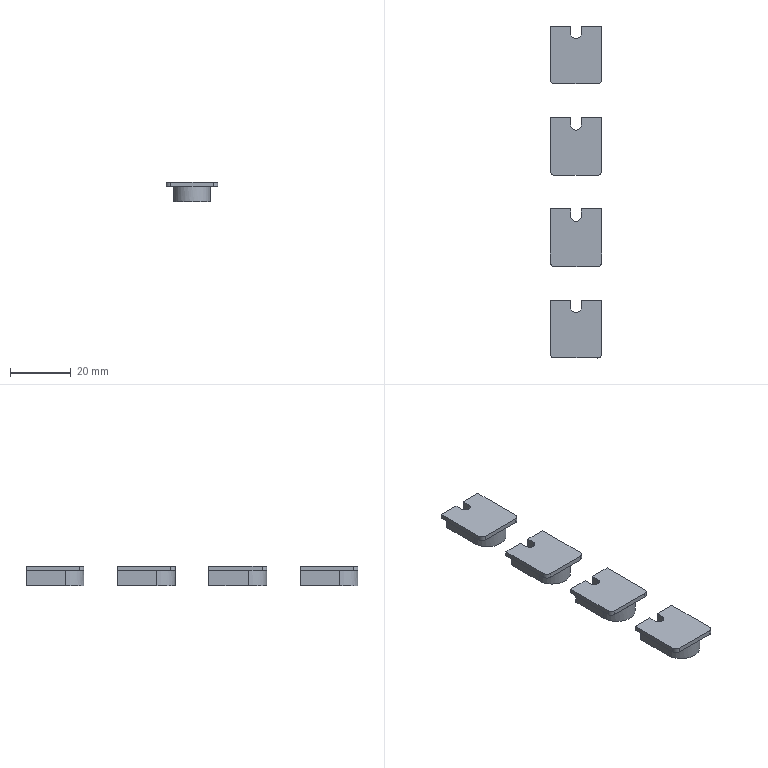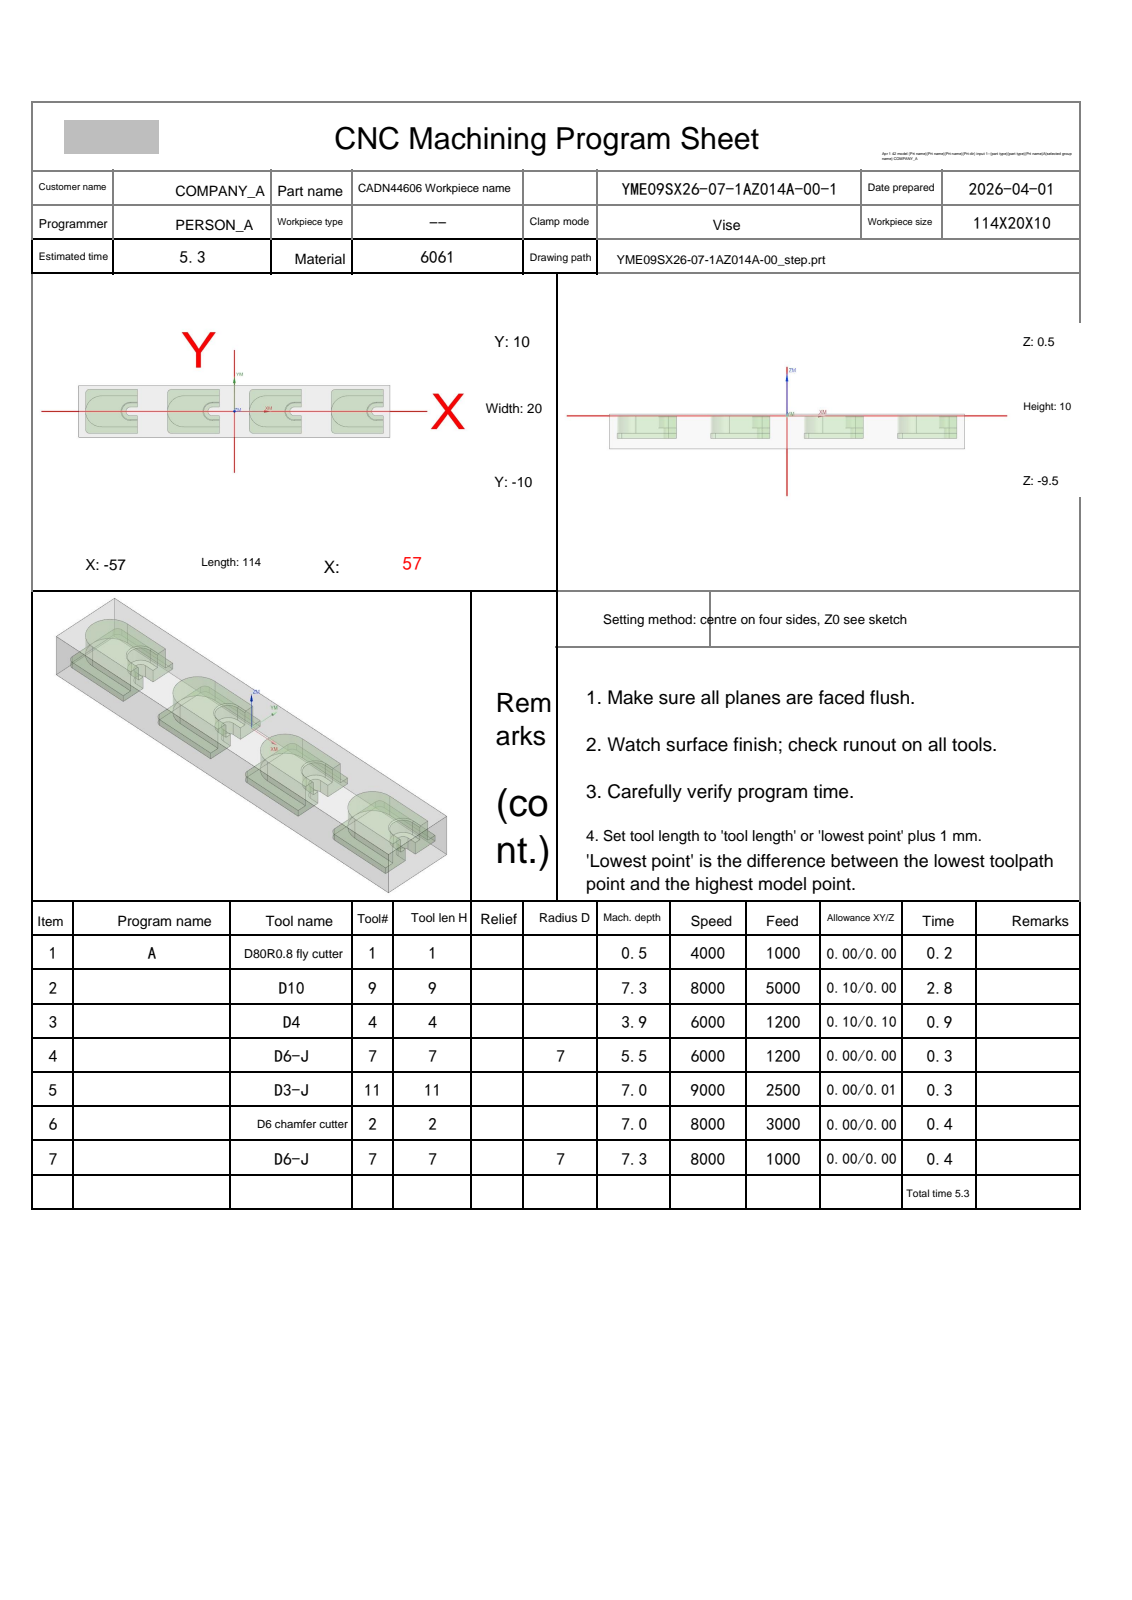NC program | NX | posted by the shop | part box 17.001 x 109 x 6.504 mm
Lines 1 to 2416 of 4321, first 1830 of 2414 lines:
%
O0001
(Machine time: 6.61 MIN)
(===Total Tool:6===)
(T1=D80R0.8 fly cutter D=80.  R=0.8  D-  H01 Z=-0.   )
(T9=D10     D=10.  R=0.   D-  H09 Z=-6.8  )
(T4=D4      D=4.   R=0.   D-  H04 Z=-3.4  )
(T7=D6-J    D=6.   R=0.   D7  H07 Z=-6.8  )
(T11=D3-J   D=3.   R=0.   D-  H11 Z=-6.45 )
(T2=D6 chamfer cutter   D=6.   R=0.   D-  H02 Z=-6.5  )
G80 G90 G17 G49 G40
G91 G28 Z0
M01
N1 T01 M06
(D80R0.8 fly cutter D=80. R=0.8 H=01 ce=0.00 di=0.00)
G00 G90 G54 X-99.5 Y.005 M03 S4000
G43 H01 Z20.
M08
Z2.
G01 Z0.0 F1000.
X-94.5
X94.5
X99.5
Z2.
G00 Z20.
G91 G28 Z0.0
M05
M09
G91 G28 Z0.0
M01
N2 T09 M06
(D10  D=10. R=0. H=09 ce=0.10 di=0.00)
G00 G90 G54 X15.75 Y13.6 M03 S8000
G43 H09 Z20.
M08
Z.5
G01 X24.5 Z.438 F5000.
G02 X29.6 Y8.5 Z.381 I0.0 J-5.1
G01 Y1.7 Z.333
G02 X29.308 Y0.0 Z.32 I-5.1 J0.0
X29.6 Y-1.7 Z.308 I-4.808 J-1.7
G01 Y-8.5 Z.26
G02 X24.5 Y-13.6 Z.203 I-5.1 J0.0
G01 X7. Z.079
G02 X.4 Y-7. Z.005 I0.0 J6.6
G01 Y7. Z-.094
G02 X7. Y13.6 Z-.168 I6.6 J0.0
G01 X24.5 Z-.292
G02 X29.6 Y8.5 Z-.349 I0.0 J-5.1
G01 Y1.7 Z-.397
G02 X29.308 Y0.0 Z-.41 I-5.1 J0.0
X29.6 Y-1.7 Z-.422 I-4.808 J-1.7
G01 Y-8.5 Z-.47
G02 X24.5 Y-13.6 Z-.527 I-5.1 J0.0
G01 X7. Z-.651
G02 X.4 Y-7. Z-.725 I0.0 J6.6
G01 Y7. Z-.824
G02 X7. Y13.6 Z-.898 I6.6 J0.0
G01 X24.5 Z-1.022
G02 X29.6 Y8.5 Z-1.079 I0.0 J-5.1
G01 Y1.7 Z-1.127
G02 X29.308 Y0.0 Z-1.14 I-5.1 J0.0
X29.6 Y-1.7 Z-1.152 I-4.808 J-1.7
G01 Y-8.5 Z-1.2
G02 X24.5 Y-13.6 Z-1.257 I-5.1 J0.0
G01 X7. Z-1.381
G02 X.4 Y-7. Z-1.455 I0.0 J6.6
G01 Y7. Z-1.554
G02 X7. Y13.6 Z-1.628 I6.6 J0.0
G01 X24.5 Z-1.752
G02 X29.6 Y8.5 Z-1.809 I0.0 J-5.1
G01 Y1.7 Z-1.857
G02 X29.308 Y0.0 Z-1.87 I-5.1 J0.0
X29.6 Y-1.7 Z-1.882 I-4.808 J-1.7
G01 Y-8.5 Z-1.93
G02 X24.5 Y-13.6 Z-1.987 I-5.1 J0.0
G01 X7. Z-2.111
G02 X.4 Y-7. Z-2.185 I0.0 J6.6
G01 Y7. Z-2.284
G02 X7. Y13.6 Z-2.358 I6.6 J0.0
G01 X24.5 Z-2.482
G02 X29.6 Y8.5 Z-2.539 I0.0 J-5.1
G01 Y1.7 Z-2.587
G02 X29.308 Y0.0 Z-2.6 I-5.1 J0.0
X29.6 Y-1.7 Z-2.612 I-4.808 J-1.7
G01 Y-8.5 Z-2.66
G02 X24.5 Y-13.6 Z-2.717 I-5.1 J0.0
G01 X7. Z-2.841
G02 X.4 Y-7. Z-2.915 I0.0 J6.6
G01 Y7. Z-3.014
G02 X7. Y13.6 Z-3.088 I6.6 J0.0
G01 X24.5 Z-3.212
G02 X29.6 Y8.5 Z-3.269 I0.0 J-5.1
G01 Y1.7 Z-3.317
G02 X29.308 Y0.0 Z-3.33 I-5.1 J0.0
X29.6 Y-1.7 Z-3.342 I-4.808 J-1.7
G01 Y-8.5 Z-3.39
G02 X24.5 Y-13.6 Z-3.447 I-5.1 J0.0
G01 X7. Z-3.571
G02 X.4 Y-7. Z-3.645 I0.0 J6.6
G01 Y7. Z-3.744
G02 X7. Y13.6 Z-3.818 I6.6 J0.0
G01 X24.5 Z-3.942
G02 X29.6 Y8.5 Z-3.999 I0.0 J-5.1
G01 Y1.7 Z-4.047
G02 X29.308 Y0.0 Z-4.06 I-5.1 J0.0
X29.6 Y-1.7 Z-4.072 I-4.808 J-1.7
G01 Y-8.5 Z-4.12
G02 X24.5 Y-13.6 Z-4.177 I-5.1 J0.0
G01 X7. Z-4.301
G02 X.4 Y-7. Z-4.375 I0.0 J6.6
G01 Y7. Z-4.474
G02 X7. Y13.6 Z-4.548 I6.6 J0.0
G01 X24.5 Z-4.672
G02 X29.6 Y8.5 Z-4.729 I0.0 J-5.1
G01 Y1.7 Z-4.777
G02 X29.308 Y0.0 Z-4.79 I-5.1 J0.0
X29.6 Y-1.7 Z-4.802 I-4.808 J-1.7
G01 Y-8.5 Z-4.85
G02 X24.5 Y-13.6 Z-4.907 I-5.1 J0.0
G01 X7. Z-5.031
G02 X.4 Y-7. Z-5.105 I0.0 J6.6
G01 Y7. Z-5.204
G02 X7. Y13.6 Z-5.278 I6.6 J0.0
G01 X24.5 Z-5.402
G02 X29.6 Y8.5 Z-5.459 I0.0 J-5.1
G01 Y1.7 Z-5.507
G02 X29.308 Y0.0 Z-5.52 I-5.1 J0.0
X29.6 Y-1.7 Z-5.532 I-4.808 J-1.7
G01 Y-8.5 Z-5.58
G02 X24.5 Y-13.6 Z-5.637 I-5.1 J0.0
G01 X7. Z-5.761
G02 X.4 Y-7. Z-5.835 I0.0 J6.6
G01 Y7. Z-5.934
G02 X7. Y13.6 Z-6.008 I6.6 J0.0
G01 X24.5 Z-6.132
G02 X29.6 Y8.5 Z-6.189 I0.0 J-5.1
G01 Y1.7 Z-6.237
G02 X29.308 Y0.0 Z-6.25 I-5.1 J0.0
X29.6 Y-1.7 Z-6.262 I-4.808 J-1.7
G01 Y-8.5 Z-6.31
G02 X24.5 Y-13.6 Z-6.367 I-5.1 J0.0
G01 X7. Z-6.491
G02 X.4 Y-7. Z-6.565 I0.0 J6.6
G01 Y7. Z-6.664
G02 X7. Y13.6 Z-6.738 I6.6 J0.0
G01 X15.75 Z-6.8
X24.5
G02 X29.6 Y8.5 I0.0 J-5.1
G01 Y1.7
G02 X29.308 Y0.0 I-5.1 J0.0
X29.6 Y-1.7 I-4.808 J-1.7
G01 Y-8.5
G02 X24.5 Y-13.6 I-5.1 J0.0
G01 X7.
G02 X.4 Y-7. I0.0 J6.6
G01 Y7.
G02 X7. Y13.6 I6.6 J0.0
G01 X15.75
X16.25
Z-5.8
G00 Z20.
X-14.25
Z.5
G01 X-5.5 Z.438
G02 X-.4 Y8.5 Z.381 I0.0 J-5.1
G01 Y1.7 Z.333
G02 X-.692 Y0.0 Z.32 I-5.1 J0.0
X-.4 Y-1.7 Z.308 I-4.808 J-1.7
G01 Y-8.5 Z.26
G02 X-5.5 Y-13.6 Z.203 I-5.1 J0.0
G01 X-23. Z.079
G02 X-29.6 Y-7. Z.005 I0.0 J6.6
G01 Y7. Z-.094
G02 X-23. Y13.6 Z-.168 I6.6 J0.0
G01 X-5.5 Z-.292
G02 X-.4 Y8.5 Z-.349 I0.0 J-5.1
G01 Y1.7 Z-.397
G02 X-.692 Y0.0 Z-.41 I-5.1 J0.0
X-.4 Y-1.7 Z-.422 I-4.808 J-1.7
G01 Y-8.5 Z-.47
G02 X-5.5 Y-13.6 Z-.527 I-5.1 J0.0
G01 X-23. Z-.651
G02 X-29.6 Y-7. Z-.725 I0.0 J6.6
G01 Y7. Z-.824
G02 X-23. Y13.6 Z-.898 I6.6 J0.0
G01 X-5.5 Z-1.022
G02 X-.4 Y8.5 Z-1.079 I0.0 J-5.1
G01 Y1.7 Z-1.127
G02 X-.692 Y0.0 Z-1.14 I-5.1 J0.0
X-.4 Y-1.7 Z-1.152 I-4.808 J-1.7
G01 Y-8.5 Z-1.2
G02 X-5.5 Y-13.6 Z-1.257 I-5.1 J0.0
G01 X-23. Z-1.381
G02 X-29.6 Y-7. Z-1.455 I0.0 J6.6
G01 Y7. Z-1.554
G02 X-23. Y13.6 Z-1.628 I6.6 J0.0
G01 X-5.5 Z-1.752
G02 X-.4 Y8.5 Z-1.809 I0.0 J-5.1
G01 Y1.7 Z-1.857
G02 X-.692 Y0.0 Z-1.87 I-5.1 J0.0
X-.4 Y-1.7 Z-1.882 I-4.808 J-1.7
G01 Y-8.5 Z-1.93
G02 X-5.5 Y-13.6 Z-1.987 I-5.1 J0.0
G01 X-23. Z-2.111
G02 X-29.6 Y-7. Z-2.185 I0.0 J6.6
G01 Y7. Z-2.284
G02 X-23. Y13.6 Z-2.358 I6.6 J0.0
G01 X-5.5 Z-2.482
G02 X-.4 Y8.5 Z-2.539 I0.0 J-5.1
G01 Y1.7 Z-2.587
G02 X-.692 Y0.0 Z-2.6 I-5.1 J0.0
X-.4 Y-1.7 Z-2.612 I-4.808 J-1.7
G01 Y-8.5 Z-2.66
G02 X-5.5 Y-13.6 Z-2.717 I-5.1 J0.0
G01 X-23. Z-2.841
G02 X-29.6 Y-7. Z-2.915 I0.0 J6.6
G01 Y7. Z-3.014
G02 X-23. Y13.6 Z-3.088 I6.6 J0.0
G01 X-5.5 Z-3.212
G02 X-.4 Y8.5 Z-3.269 I0.0 J-5.1
G01 Y1.7 Z-3.317
G02 X-.692 Y0.0 Z-3.33 I-5.1 J0.0
X-.4 Y-1.7 Z-3.342 I-4.808 J-1.7
G01 Y-8.5 Z-3.39
G02 X-5.5 Y-13.6 Z-3.447 I-5.1 J0.0
G01 X-23. Z-3.571
G02 X-29.6 Y-7. Z-3.645 I0.0 J6.6
G01 Y7. Z-3.744
G02 X-23. Y13.6 Z-3.818 I6.6 J0.0
G01 X-5.5 Z-3.942
G02 X-.4 Y8.5 Z-3.999 I0.0 J-5.1
G01 Y1.7 Z-4.047
G02 X-.692 Y0.0 Z-4.06 I-5.1 J0.0
X-.4 Y-1.7 Z-4.072 I-4.808 J-1.7
G01 Y-8.5 Z-4.12
G02 X-5.5 Y-13.6 Z-4.177 I-5.1 J0.0
G01 X-23. Z-4.301
G02 X-29.6 Y-7. Z-4.375 I0.0 J6.6
G01 Y7. Z-4.474
G02 X-23. Y13.6 Z-4.548 I6.6 J0.0
G01 X-5.5 Z-4.672
G02 X-.4 Y8.5 Z-4.729 I0.0 J-5.1
G01 Y1.7 Z-4.777
G02 X-.692 Y0.0 Z-4.79 I-5.1 J0.0
X-.4 Y-1.7 Z-4.802 I-4.808 J-1.7
G01 Y-8.5 Z-4.85
G02 X-5.5 Y-13.6 Z-4.907 I-5.1 J0.0
G01 X-23. Z-5.031
G02 X-29.6 Y-7. Z-5.105 I0.0 J6.6
G01 Y7. Z-5.204
G02 X-23. Y13.6 Z-5.278 I6.6 J0.0
G01 X-5.5 Z-5.402
G02 X-.4 Y8.5 Z-5.459 I0.0 J-5.1
G01 Y1.7 Z-5.507
G02 X-.692 Y0.0 Z-5.52 I-5.1 J0.0
X-.4 Y-1.7 Z-5.532 I-4.808 J-1.7
G01 Y-8.5 Z-5.58
G02 X-5.5 Y-13.6 Z-5.637 I-5.1 J0.0
G01 X-23. Z-5.761
G02 X-29.6 Y-7. Z-5.835 I0.0 J6.6
G01 Y7. Z-5.934
G02 X-23. Y13.6 Z-6.008 I6.6 J0.0
G01 X-5.5 Z-6.132
G02 X-.4 Y8.5 Z-6.189 I0.0 J-5.1
G01 Y1.7 Z-6.237
G02 X-.692 Y0.0 Z-6.25 I-5.1 J0.0
X-.4 Y-1.7 Z-6.262 I-4.808 J-1.7
G01 Y-8.5 Z-6.31
G02 X-5.5 Y-13.6 Z-6.367 I-5.1 J0.0
G01 X-23. Z-6.491
G02 X-29.6 Y-7. Z-6.565 I0.0 J6.6
G01 Y7. Z-6.664
G02 X-23. Y13.6 Z-6.738 I6.6 J0.0
G01 X-14.25 Z-6.8
X-5.5
G02 X-.4 Y8.5 I0.0 J-5.1
G01 Y1.7
G02 X-.692 Y0.0 I-5.1 J0.0
X-.4 Y-1.7 I-4.808 J-1.7
G01 Y-8.5
G02 X-5.5 Y-13.6 I-5.1 J0.0
G01 X-23.
G02 X-29.6 Y-7. I0.0 J6.6
G01 Y7.
G02 X-23. Y13.6 I6.6 J0.0
G01 X-14.25
X-13.75
Z-5.8
G00 Z20.
X-44.25
Z.5
G01 X-35.5 Z.438
G02 X-30.4 Y8.5 Z.381 I0.0 J-5.1
G01 Y1.7 Z.333
G02 X-30.692 Y0.0 Z.32 I-5.1 J0.0
X-30.4 Y-1.7 Z.308 I-4.808 J-1.7
G01 Y-8.5 Z.26
G02 X-35.5 Y-13.6 Z.203 I-5.1 J0.0
G01 X-53. Z.079
G02 X-59.6 Y-7. Z.005 I0.0 J6.6
G01 Y7. Z-.094
G02 X-53. Y13.6 Z-.168 I6.6 J0.0
G01 X-35.5 Z-.292
G02 X-30.4 Y8.5 Z-.349 I0.0 J-5.1
G01 Y1.7 Z-.397
G02 X-30.692 Y0.0 Z-.41 I-5.1 J0.0
X-30.4 Y-1.7 Z-.422 I-4.808 J-1.7
G01 Y-8.5 Z-.47
G02 X-35.5 Y-13.6 Z-.527 I-5.1 J0.0
G01 X-53. Z-.651
G02 X-59.6 Y-7. Z-.725 I0.0 J6.6
G01 Y7. Z-.824
G02 X-53. Y13.6 Z-.898 I6.6 J0.0
G01 X-35.5 Z-1.022
G02 X-30.4 Y8.5 Z-1.079 I0.0 J-5.1
G01 Y1.7 Z-1.127
G02 X-30.692 Y0.0 Z-1.14 I-5.1 J0.0
X-30.4 Y-1.7 Z-1.152 I-4.808 J-1.7
G01 Y-8.5 Z-1.2
G02 X-35.5 Y-13.6 Z-1.257 I-5.1 J0.0
G01 X-53. Z-1.381
G02 X-59.6 Y-7. Z-1.455 I0.0 J6.6
G01 Y7. Z-1.554
G02 X-53. Y13.6 Z-1.628 I6.6 J0.0
G01 X-35.5 Z-1.752
G02 X-30.4 Y8.5 Z-1.809 I0.0 J-5.1
G01 Y1.7 Z-1.857
G02 X-30.692 Y0.0 Z-1.87 I-5.1 J0.0
X-30.4 Y-1.7 Z-1.882 I-4.808 J-1.7
G01 Y-8.5 Z-1.93
G02 X-35.5 Y-13.6 Z-1.987 I-5.1 J0.0
G01 X-53. Z-2.111
G02 X-59.6 Y-7. Z-2.185 I0.0 J6.6
G01 Y7. Z-2.284
G02 X-53. Y13.6 Z-2.358 I6.6 J0.0
G01 X-35.5 Z-2.482
G02 X-30.4 Y8.5 Z-2.539 I0.0 J-5.1
G01 Y1.7 Z-2.587
G02 X-30.692 Y0.0 Z-2.6 I-5.1 J0.0
X-30.4 Y-1.7 Z-2.612 I-4.808 J-1.7
G01 Y-8.5 Z-2.66
G02 X-35.5 Y-13.6 Z-2.717 I-5.1 J0.0
G01 X-53. Z-2.841
G02 X-59.6 Y-7. Z-2.915 I0.0 J6.6
G01 Y7. Z-3.014
G02 X-53. Y13.6 Z-3.088 I6.6 J0.0
G01 X-35.5 Z-3.212
G02 X-30.4 Y8.5 Z-3.269 I0.0 J-5.1
G01 Y1.7 Z-3.317
G02 X-30.692 Y0.0 Z-3.33 I-5.1 J0.0
X-30.4 Y-1.7 Z-3.342 I-4.808 J-1.7
G01 Y-8.5 Z-3.39
G02 X-35.5 Y-13.6 Z-3.447 I-5.1 J0.0
G01 X-53. Z-3.571
G02 X-59.6 Y-7. Z-3.645 I0.0 J6.6
G01 Y7. Z-3.744
G02 X-53. Y13.6 Z-3.818 I6.6 J0.0
G01 X-35.5 Z-3.942
G02 X-30.4 Y8.5 Z-3.999 I0.0 J-5.1
G01 Y1.7 Z-4.047
G02 X-30.692 Y0.0 Z-4.06 I-5.1 J0.0
X-30.4 Y-1.7 Z-4.072 I-4.808 J-1.7
G01 Y-8.5 Z-4.12
G02 X-35.5 Y-13.6 Z-4.177 I-5.1 J0.0
G01 X-53. Z-4.301
G02 X-59.6 Y-7. Z-4.375 I0.0 J6.6
G01 Y7. Z-4.474
G02 X-53. Y13.6 Z-4.548 I6.6 J0.0
G01 X-35.5 Z-4.672
G02 X-30.4 Y8.5 Z-4.729 I0.0 J-5.1
G01 Y1.7 Z-4.777
G02 X-30.692 Y0.0 Z-4.79 I-5.1 J0.0
X-30.4 Y-1.7 Z-4.802 I-4.808 J-1.7
G01 Y-8.5 Z-4.85
G02 X-35.5 Y-13.6 Z-4.907 I-5.1 J0.0
G01 X-53. Z-5.031
G02 X-59.6 Y-7. Z-5.105 I0.0 J6.6
G01 Y7. Z-5.204
G02 X-53. Y13.6 Z-5.278 I6.6 J0.0
G01 X-35.5 Z-5.402
G02 X-30.4 Y8.5 Z-5.459 I0.0 J-5.1
G01 Y1.7 Z-5.507
G02 X-30.692 Y0.0 Z-5.52 I-5.1 J0.0
X-30.4 Y-1.7 Z-5.532 I-4.808 J-1.7
G01 Y-8.5 Z-5.58
G02 X-35.5 Y-13.6 Z-5.637 I-5.1 J0.0
G01 X-53. Z-5.761
G02 X-59.6 Y-7. Z-5.835 I0.0 J6.6
G01 Y7. Z-5.934
G02 X-53. Y13.6 Z-6.008 I6.6 J0.0
G01 X-35.5 Z-6.132
G02 X-30.4 Y8.5 Z-6.189 I0.0 J-5.1
G01 Y1.7 Z-6.237
G02 X-30.692 Y0.0 Z-6.25 I-5.1 J0.0
X-30.4 Y-1.7 Z-6.262 I-4.808 J-1.7
G01 Y-8.5 Z-6.31
G02 X-35.5 Y-13.6 Z-6.367 I-5.1 J0.0
G01 X-53. Z-6.491
G02 X-59.6 Y-7. Z-6.565 I0.0 J6.6
G01 Y7. Z-6.664
G02 X-53. Y13.6 Z-6.738 I6.6 J0.0
G01 X-44.25 Z-6.8
X-35.5
G02 X-30.4 Y8.5 I0.0 J-5.1
G01 Y1.7
G02 X-30.692 Y0.0 I-5.1 J0.0
X-30.4 Y-1.7 I-4.808 J-1.7
G01 Y-8.5
G02 X-35.5 Y-13.6 I-5.1 J0.0
G01 X-53.
G02 X-59.6 Y-7. I0.0 J6.6
G01 Y7.
G02 X-53. Y13.6 I6.6 J0.0
G01 X-44.25
X-43.75
Z-5.8
G00 Z20.
X45.75
Z.5
G01 X54.5 Z.438
G02 X59.6 Y8.5 Z.381 I0.0 J-5.1
G01 Y1.7 Z.333
G02 X59.308 Y0.0 Z.32 I-5.1 J0.0
X59.6 Y-1.7 Z.308 I-4.808 J-1.7
G01 Y-8.5 Z.26
G02 X54.5 Y-13.6 Z.203 I-5.1 J0.0
G01 X37. Z.079
G02 X30.4 Y-7. Z.005 I0.0 J6.6
G01 Y7. Z-.094
G02 X37. Y13.6 Z-.168 I6.6 J0.0
G01 X54.5 Z-.292
G02 X59.6 Y8.5 Z-.349 I0.0 J-5.1
G01 Y1.7 Z-.397
G02 X59.308 Y0.0 Z-.41 I-5.1 J0.0
X59.6 Y-1.7 Z-.422 I-4.808 J-1.7
G01 Y-8.5 Z-.47
G02 X54.5 Y-13.6 Z-.527 I-5.1 J0.0
G01 X37. Z-.651
G02 X30.4 Y-7. Z-.725 I0.0 J6.6
G01 Y7. Z-.824
G02 X37. Y13.6 Z-.898 I6.6 J0.0
G01 X54.5 Z-1.022
G02 X59.6 Y8.5 Z-1.079 I0.0 J-5.1
G01 Y1.7 Z-1.127
G02 X59.308 Y0.0 Z-1.14 I-5.1 J0.0
X59.6 Y-1.7 Z-1.152 I-4.808 J-1.7
G01 Y-8.5 Z-1.2
G02 X54.5 Y-13.6 Z-1.257 I-5.1 J0.0
G01 X37. Z-1.381
G02 X30.4 Y-7. Z-1.455 I0.0 J6.6
G01 Y7. Z-1.554
G02 X37. Y13.6 Z-1.628 I6.6 J0.0
G01 X54.5 Z-1.752
G02 X59.6 Y8.5 Z-1.809 I0.0 J-5.1
G01 Y1.7 Z-1.857
G02 X59.308 Y0.0 Z-1.87 I-5.1 J0.0
X59.6 Y-1.7 Z-1.882 I-4.808 J-1.7
G01 Y-8.5 Z-1.93
G02 X54.5 Y-13.6 Z-1.987 I-5.1 J0.0
G01 X37. Z-2.111
G02 X30.4 Y-7. Z-2.185 I0.0 J6.6
G01 Y7. Z-2.284
G02 X37. Y13.6 Z-2.358 I6.6 J0.0
G01 X54.5 Z-2.482
G02 X59.6 Y8.5 Z-2.539 I0.0 J-5.1
G01 Y1.7 Z-2.587
G02 X59.308 Y0.0 Z-2.6 I-5.1 J0.0
X59.6 Y-1.7 Z-2.612 I-4.808 J-1.7
G01 Y-8.5 Z-2.66
G02 X54.5 Y-13.6 Z-2.717 I-5.1 J0.0
G01 X37. Z-2.841
G02 X30.4 Y-7. Z-2.915 I0.0 J6.6
G01 Y7. Z-3.014
G02 X37. Y13.6 Z-3.088 I6.6 J0.0
G01 X54.5 Z-3.212
G02 X59.6 Y8.5 Z-3.269 I0.0 J-5.1
G01 Y1.7 Z-3.317
G02 X59.308 Y0.0 Z-3.33 I-5.1 J0.0
X59.6 Y-1.7 Z-3.342 I-4.808 J-1.7
G01 Y-8.5 Z-3.39
G02 X54.5 Y-13.6 Z-3.447 I-5.1 J0.0
G01 X37. Z-3.571
G02 X30.4 Y-7. Z-3.645 I0.0 J6.6
G01 Y7. Z-3.744
G02 X37. Y13.6 Z-3.818 I6.6 J0.0
G01 X54.5 Z-3.942
G02 X59.6 Y8.5 Z-3.999 I0.0 J-5.1
G01 Y1.7 Z-4.047
G02 X59.308 Y0.0 Z-4.06 I-5.1 J0.0
X59.6 Y-1.7 Z-4.072 I-4.808 J-1.7
G01 Y-8.5 Z-4.12
G02 X54.5 Y-13.6 Z-4.177 I-5.1 J0.0
G01 X37. Z-4.301
G02 X30.4 Y-7. Z-4.375 I0.0 J6.6
G01 Y7. Z-4.474
G02 X37. Y13.6 Z-4.548 I6.6 J0.0
G01 X54.5 Z-4.672
G02 X59.6 Y8.5 Z-4.729 I0.0 J-5.1
G01 Y1.7 Z-4.777
G02 X59.308 Y0.0 Z-4.79 I-5.1 J0.0
X59.6 Y-1.7 Z-4.802 I-4.808 J-1.7
G01 Y-8.5 Z-4.85
G02 X54.5 Y-13.6 Z-4.907 I-5.1 J0.0
G01 X37. Z-5.031
G02 X30.4 Y-7. Z-5.105 I0.0 J6.6
G01 Y7. Z-5.204
G02 X37. Y13.6 Z-5.278 I6.6 J0.0
G01 X54.5 Z-5.402
G02 X59.6 Y8.5 Z-5.459 I0.0 J-5.1
G01 Y1.7 Z-5.507
G02 X59.308 Y0.0 Z-5.52 I-5.1 J0.0
X59.6 Y-1.7 Z-5.532 I-4.808 J-1.7
G01 Y-8.5 Z-5.58
G02 X54.5 Y-13.6 Z-5.637 I-5.1 J0.0
G01 X37. Z-5.761
G02 X30.4 Y-7. Z-5.835 I0.0 J6.6
G01 Y7. Z-5.934
G02 X37. Y13.6 Z-6.008 I6.6 J0.0
G01 X54.5 Z-6.132
G02 X59.6 Y8.5 Z-6.189 I0.0 J-5.1
G01 Y1.7 Z-6.237
G02 X59.308 Y0.0 Z-6.25 I-5.1 J0.0
X59.6 Y-1.7 Z-6.262 I-4.808 J-1.7
G01 Y-8.5 Z-6.31
G02 X54.5 Y-13.6 Z-6.367 I-5.1 J0.0
G01 X37. Z-6.491
G02 X30.4 Y-7. Z-6.565 I0.0 J6.6
G01 Y7. Z-6.664
G02 X37. Y13.6 Z-6.738 I6.6 J0.0
G01 X45.75 Z-6.8
X54.5
G02 X59.6 Y8.5 I0.0 J-5.1
G01 Y1.7
G02 X59.308 Y0.0 I-5.1 J0.0
X59.6 Y-1.7 I-4.808 J-1.7
G01 Y-8.5
G02 X54.5 Y-13.6 I-5.1 J0.0
G01 X37.
G02 X30.4 Y-7. I0.0 J6.6
G01 Y7.
G02 X37. Y13.6 I6.6 J0.0
G01 X45.75
X46.25
Z-5.8
G00 Z20.
G00 G90 X-11.8 Y16.5 M03 S8000
Z10.5
Z.956
G01 Z-.544 F4000.
Y13.4
X-.6
Y13.291
X5.26 Y13.159
X5.275 Y13.163
G02 X7. Y13.4 I1.725 J-6.163
G01 X29.4
Y13.291
X35.26 Y13.159
X35.275 Y13.163
G02 X37. Y13.4 I1.725 J-6.163
G01 X59.4
Y11.1
X41.5
G03 X31.1 Y3.879 I0.0 J-11.1
G01 Y11.1
G03 X29.6 Y12.6 I-1.5 J0.0
G01 X11.5
G03 X1.1 Y7.113 I0.0 J-12.6
G01 Y11.1
G03 X-.4 Y12.6 I-1.5 J0.0
G01 X-18.5
G03 X-30.4 Y4.141 I0.0 J-12.6
G01 Y11.1
X-48.5
G03 X-59.4 Y2.098 I0.0 J-11.1
G01 Y4.899
Y7.
G02 X-53. Y13.4 I6.4 J0.0
G01 X-30.6
Y13.291
X-24.739 Y13.159
X-24.725 Y13.163
G02 X-23. Y13.4 I1.725 J-6.163
G01 X-11.8
X-11.3
Y16.5
Z.956
G00 Z10.5
X48.2 Y-16.5
Z.956
G01 Z-.544
Y-13.4
X37.
G02 X35.26 Y-13.159 I0.0 J6.4
G01 X29.4 Y-13.291
Y-13.4
X7.
G02 X5.26 Y-13.159 I0.0 J6.4
G01 X-.6 Y-13.291
Y-13.4
X-23.
G02 X-24.74 Y-13.159 I0.0 J6.4
G01 X-30.6 Y-13.291
Y-13.4
X-53.
G02 X-59.4 Y-7. I0.0 J6.4
G01 Y-4.903
Y-2.097
G03 X-48.5 Y-11.1 I10.9 J2.097
G01 X-30.4
Y-4.141
G03 X-18.5 Y-12.6 I11.9 J4.141
G01 X-.4
G03 X1.1 Y-11.1 I0.0 J1.5
G01 Y-7.641
G03 X.623 Y-6.887 I-.835 J0.0
G01 X.243 Y-6.707
X.05 Y-6.663
G03 X-.4 Y-7.113 I0.0 J-.45
G01 Y-11.1
X-18.5
G02 X-29.6 Y0.0 I0.0 J11.1
X-18.5 Y11.1 I11.1 J0.0
G01 X-.4
Y-7.113
G03 X.532 Y-8.045 I.932 J0.0
X.869 Y-7.982 I0.0 J.932
G02 X1.23 Y-7.915 I.361 J-.933
X1.984 Y-8.259 I0.0 J-1.
G03 X11.5 Y-12.6 I9.516 J8.259
G01 X29.6
G03 X31.1 Y-11.1 I0.0 J1.5
G01 Y-4.407
G03 X30.623 Y-3.653 I-.835 J0.0
G01 X30.243 Y-3.473
X30.05 Y-3.429
G03 X29.6 Y-3.879 I0.0 J-.45
G01 Y-11.1
X11.5
G02 X.4 Y0.0 I0.0 J11.1
X11.5 Y11.1 I11.1 J0.0
G01 X29.6
Y-3.879
G03 X29.774 Y-4.235 I.45 J0.0
X30.019 Y-4.319 I.245 J.316
X30.338 Y-4.161 I0.0 J.4
G01 X30.607 Y-3.807
G02 X30.833 Y-3.694 I.227 J-.172
X31.1 Y-3.879 I0.0 J-.285
G03 X41.5 Y-11.1 I10.4 J3.879
G01 X59.4
Y-13.4
X48.2
X47.7
Y-16.5
Z.956
G00 Z10.5
X-11.8 Y16.5
Z.411
G01 Z-1.089
Y13.4
X-.6
Y13.291
X5.26 Y13.159
X5.275 Y13.163
G02 X7. Y13.4 I1.725 J-6.163
G01 X29.4
Y13.291
X35.26 Y13.159
X35.275 Y13.163
G02 X37. Y13.4 I1.725 J-6.163
G01 X59.4
Y11.1
X41.5
G03 X31.1 Y3.879 I0.0 J-11.1
G01 Y11.1
G03 X29.6 Y12.6 I-1.5 J0.0
G01 X11.5
G03 X1.1 Y7.113 I0.0 J-12.6
G01 Y11.1
G03 X-.4 Y12.6 I-1.5 J0.0
G01 X-18.5
G03 X-30.4 Y4.141 I0.0 J-12.6
G01 Y11.1
X-48.5
G03 X-59.4 Y2.098 I0.0 J-11.1
G01 Y4.899
Y7.
G02 X-53. Y13.4 I6.4 J0.0
G01 X-30.6
Y13.291
X-24.739 Y13.159
X-24.725 Y13.163
G02 X-23. Y13.4 I1.725 J-6.163
G01 X-11.8
X-11.3
Y16.5
Z.411
G00 Z10.5
X48.2 Y-16.5
Z.411
G01 Z-1.089
Y-13.4
X37.
G02 X35.26 Y-13.159 I0.0 J6.4
G01 X29.4 Y-13.291
Y-13.4
X7.
G02 X5.26 Y-13.159 I0.0 J6.4
G01 X-.6 Y-13.291
Y-13.4
X-23.
G02 X-24.74 Y-13.159 I0.0 J6.4
G01 X-30.6 Y-13.291
Y-13.4
X-53.
G02 X-59.4 Y-7. I0.0 J6.4
G01 Y-4.903
Y-2.097
G03 X-48.5 Y-11.1 I10.9 J2.097
G01 X-30.4
Y-4.141
G03 X-18.5 Y-12.6 I11.9 J4.141
G01 X-.4
G03 X1.1 Y-11.1 I0.0 J1.5
G01 Y-7.641
G03 X.623 Y-6.887 I-.835 J0.0
G01 X.243 Y-6.707
X.05 Y-6.663
G03 X-.4 Y-7.113 I0.0 J-.45
G01 Y-11.1
X-18.5
G02 X-29.6 Y0.0 I0.0 J11.1
X-18.5 Y11.1 I11.1 J0.0
G01 X-.4
Y-7.113
G03 X.532 Y-8.045 I.932 J0.0
X.869 Y-7.982 I0.0 J.932
G02 X1.23 Y-7.915 I.361 J-.933
X1.984 Y-8.259 I0.0 J-1.
G03 X11.5 Y-12.6 I9.516 J8.259
G01 X29.6
G03 X31.1 Y-11.1 I0.0 J1.5
G01 Y-4.407
G03 X30.623 Y-3.653 I-.835 J0.0
G01 X30.243 Y-3.473
X30.05 Y-3.429
G03 X29.6 Y-3.879 I0.0 J-.45
G01 Y-11.1
X11.5
G02 X.4 Y0.0 I0.0 J11.1
X11.5 Y11.1 I11.1 J0.0
G01 X29.6
Y-3.879
G03 X29.774 Y-4.235 I.45 J0.0
X30.019 Y-4.319 I.245 J.316
X30.338 Y-4.161 I0.0 J.4
G01 X30.607 Y-3.807
G02 X30.833 Y-3.694 I.227 J-.172
X31.1 Y-3.879 I0.0 J-.285
G03 X41.5 Y-11.1 I10.4 J3.879
G01 X59.4
Y-13.4
X48.2
X47.7
Y-16.5
Z.411
G00 Z10.5
X-11.8 Y16.5
Z-.133
G01 Z-1.633
Y13.4
X-.6
Y13.291
X5.26 Y13.159
X5.275 Y13.163
G02 X7. Y13.4 I1.725 J-6.163
G01 X29.4
Y13.291
X35.26 Y13.159
X35.275 Y13.163
G02 X37. Y13.4 I1.725 J-6.163
G01 X59.4
Y11.1
X41.5
G03 X31.1 Y3.879 I0.0 J-11.1
G01 Y11.1
G03 X29.6 Y12.6 I-1.5 J0.0
G01 X11.5
G03 X1.1 Y7.113 I0.0 J-12.6
G01 Y11.1
G03 X-.4 Y12.6 I-1.5 J0.0
G01 X-18.5
G03 X-30.4 Y4.141 I0.0 J-12.6
G01 Y11.1
X-48.5
G03 X-59.4 Y2.098 I0.0 J-11.1
G01 Y4.899
Y7.
G02 X-53. Y13.4 I6.4 J0.0
G01 X-30.6
Y13.291
X-24.739 Y13.159
X-24.725 Y13.163
G02 X-23. Y13.4 I1.725 J-6.163
G01 X-11.8
X-11.3
Y16.5
Z-.133
G00 Z10.5
X48.2 Y-16.5
Z-.133
G01 Z-1.633
Y-13.4
X37.
G02 X35.26 Y-13.159 I0.0 J6.4
G01 X29.4 Y-13.291
Y-13.4
X7.
G02 X5.26 Y-13.159 I0.0 J6.4
G01 X-.6 Y-13.291
Y-13.4
X-23.
G02 X-24.74 Y-13.159 I0.0 J6.4
G01 X-30.6 Y-13.291
Y-13.4
X-53.
G02 X-59.4 Y-7. I0.0 J6.4
G01 Y-4.903
Y-2.097
G03 X-48.5 Y-11.1 I10.9 J2.097
G01 X-30.4
Y-4.141
G03 X-18.5 Y-12.6 I11.9 J4.141
G01 X-.4
G03 X1.1 Y-11.1 I0.0 J1.5
G01 Y-7.641
G03 X.623 Y-6.887 I-.835 J0.0
G01 X.243 Y-6.707
X.05 Y-6.663
G03 X-.4 Y-7.113 I0.0 J-.45
G01 Y-11.1
X-18.5
G02 X-29.6 Y0.0 I0.0 J11.1
X-18.5 Y11.1 I11.1 J0.0
G01 X-.4
Y-7.113
G03 X.532 Y-8.045 I.932 J0.0
X.869 Y-7.982 I0.0 J.932
G02 X1.23 Y-7.915 I.361 J-.933
X1.984 Y-8.259 I0.0 J-1.
G03 X11.5 Y-12.6 I9.516 J8.259
G01 X29.6
G03 X31.1 Y-11.1 I0.0 J1.5
G01 Y-4.407
G03 X30.623 Y-3.653 I-.835 J0.0
G01 X30.243 Y-3.473
X30.05 Y-3.429
G03 X29.6 Y-3.879 I0.0 J-.45
G01 Y-11.1
X11.5
G02 X.4 Y0.0 I0.0 J11.1
X11.5 Y11.1 I11.1 J0.0
G01 X29.6
Y-3.879
G03 X29.774 Y-4.235 I.45 J0.0
X30.019 Y-4.319 I.245 J.316
X30.338 Y-4.161 I0.0 J.4
G01 X30.607 Y-3.807
G02 X30.833 Y-3.694 I.227 J-.172
X31.1 Y-3.879 I0.0 J-.285
G03 X41.5 Y-11.1 I10.4 J3.879
G01 X59.4
Y-13.4
X48.2
X47.7
Y-16.5
Z-.133
G00 Z10.5
X-11.8 Y16.5
Z-.678
G01 Z-2.178
Y13.4
X-.6
Y13.291
X5.26 Y13.159
X5.275 Y13.163
G02 X7. Y13.4 I1.725 J-6.163
G01 X29.4
Y13.291
X35.26 Y13.159
X35.275 Y13.163
G02 X37. Y13.4 I1.725 J-6.163
G01 X59.4
Y11.1
X41.5
G03 X31.1 Y3.879 I0.0 J-11.1
G01 Y11.1
G03 X29.6 Y12.6 I-1.5 J0.0
G01 X11.5
G03 X1.1 Y7.113 I0.0 J-12.6
G01 Y11.1
G03 X-.4 Y12.6 I-1.5 J0.0
G01 X-18.5
G03 X-30.4 Y4.141 I0.0 J-12.6
G01 Y11.1
X-48.5
G03 X-59.4 Y2.098 I0.0 J-11.1
G01 Y4.899
Y7.
G02 X-53. Y13.4 I6.4 J0.0
G01 X-30.6
Y13.291
X-24.739 Y13.159
X-24.725 Y13.163
G02 X-23. Y13.4 I1.725 J-6.163
G01 X-11.8
X-11.3
Y16.5
Z-.678
G00 Z10.5
X48.2 Y-16.5
Z-.678
G01 Z-2.178
Y-13.4
X37.
G02 X35.26 Y-13.159 I0.0 J6.4
G01 X29.4 Y-13.291
Y-13.4
X7.
G02 X5.26 Y-13.159 I0.0 J6.4
G01 X-.6 Y-13.291
Y-13.4
X-23.
G02 X-24.74 Y-13.159 I0.0 J6.4
G01 X-30.6 Y-13.291
Y-13.4
X-53.
G02 X-59.4 Y-7. I0.0 J6.4
G01 Y-4.903
Y-2.097
G03 X-48.5 Y-11.1 I10.9 J2.097
G01 X-30.4
Y-4.141
G03 X-18.5 Y-12.6 I11.9 J4.141
G01 X-.4
G03 X1.1 Y-11.1 I0.0 J1.5
G01 Y-7.641
G03 X.623 Y-6.887 I-.835 J0.0
G01 X.243 Y-6.707
X.05 Y-6.663
G03 X-.4 Y-7.113 I0.0 J-.45
G01 Y-11.1
X-18.5
G02 X-29.6 Y0.0 I0.0 J11.1
X-18.5 Y11.1 I11.1 J0.0
G01 X-.4
Y-7.113
G03 X.532 Y-8.045 I.932 J0.0
X.869 Y-7.982 I0.0 J.932
G02 X1.23 Y-7.915 I.361 J-.933
X1.984 Y-8.259 I0.0 J-1.
G03 X11.5 Y-12.6 I9.516 J8.259
G01 X29.6
G03 X31.1 Y-11.1 I0.0 J1.5
G01 Y-4.407
G03 X30.623 Y-3.653 I-.835 J0.0
G01 X30.243 Y-3.473
X30.05 Y-3.429
G03 X29.6 Y-3.879 I0.0 J-.45
G01 Y-11.1
X11.5
G02 X.4 Y0.0 I0.0 J11.1
X11.5 Y11.1 I11.1 J0.0
G01 X29.6
Y-3.879
G03 X29.774 Y-4.235 I.45 J0.0
X30.019 Y-4.319 I.245 J.316
X30.338 Y-4.161 I0.0 J.4
G01 X30.607 Y-3.807
G02 X30.833 Y-3.694 I.227 J-.172
X31.1 Y-3.879 I0.0 J-.285
G03 X41.5 Y-11.1 I10.4 J3.879
G01 X59.4
Y-13.4
X48.2
X47.7
Y-16.5
Z-.678
G00 Z10.5
X-11.8 Y16.5
Z-1.222
G01 Z-2.722
Y13.4
X-.6
Y13.291
X5.26 Y13.159
X5.275 Y13.163
G02 X7. Y13.4 I1.725 J-6.163
G01 X29.4
Y13.291
X35.26 Y13.159
X35.275 Y13.163
G02 X37. Y13.4 I1.725 J-6.163
G01 X59.4
Y11.1
X41.5
G03 X31.1 Y3.879 I0.0 J-11.1
G01 Y11.1
G03 X29.6 Y12.6 I-1.5 J0.0
G01 X11.5
G03 X1.1 Y7.113 I0.0 J-12.6
G01 Y11.1
G03 X-.4 Y12.6 I-1.5 J0.0
G01 X-18.5
G03 X-30.4 Y4.141 I0.0 J-12.6
G01 Y11.1
X-48.5
G03 X-59.4 Y2.098 I0.0 J-11.1
G01 Y4.899
Y7.
G02 X-53. Y13.4 I6.4 J0.0
G01 X-30.6
Y13.291
X-24.739 Y13.159
X-24.725 Y13.163
G02 X-23. Y13.4 I1.725 J-6.163
G01 X-11.8
X-11.3
Y16.5
Z-1.222
G00 Z10.5
X48.2 Y-16.5
Z-1.222
G01 Z-2.722
Y-13.4
X37.
G02 X35.26 Y-13.159 I0.0 J6.4
G01 X29.4 Y-13.291
Y-13.4
X7.
G02 X5.26 Y-13.159 I0.0 J6.4
G01 X-.6 Y-13.291
Y-13.4
X-23.
G02 X-24.74 Y-13.159 I0.0 J6.4
G01 X-30.6 Y-13.291
Y-13.4
X-53.
G02 X-59.4 Y-7. I0.0 J6.4
G01 Y-4.903
Y-2.097
G03 X-48.5 Y-11.1 I10.9 J2.097
G01 X-30.4
Y-4.141
G03 X-18.5 Y-12.6 I11.9 J4.141
G01 X-.4
G03 X1.1 Y-11.1 I0.0 J1.5
G01 Y-7.641
G03 X.623 Y-6.887 I-.835 J0.0
G01 X.243 Y-6.707
X.05 Y-6.663
G03 X-.4 Y-7.113 I0.0 J-.45
G01 Y-11.1
X-18.5
G02 X-29.6 Y0.0 I0.0 J11.1
X-18.5 Y11.1 I11.1 J0.0
G01 X-.4
Y-7.113
G03 X.532 Y-8.045 I.932 J0.0
X.869 Y-7.982 I0.0 J.932
G02 X1.23 Y-7.915 I.361 J-.933
X1.984 Y-8.259 I0.0 J-1.
G03 X11.5 Y-12.6 I9.516 J8.259
G01 X29.6
G03 X31.1 Y-11.1 I0.0 J1.5
G01 Y-4.407
G03 X30.623 Y-3.653 I-.835 J0.0
G01 X30.243 Y-3.473
X30.05 Y-3.429
G03 X29.6 Y-3.879 I0.0 J-.45
G01 Y-11.1
X11.5
G02 X.4 Y0.0 I0.0 J11.1
X11.5 Y11.1 I11.1 J0.0
G01 X29.6
Y-3.879
G03 X29.774 Y-4.235 I.45 J0.0
X30.019 Y-4.319 I.245 J.316
X30.338 Y-4.161 I0.0 J.4
G01 X30.607 Y-3.807
G02 X30.833 Y-3.694 I.227 J-.172
X31.1 Y-3.879 I0.0 J-.285
G03 X41.5 Y-11.1 I10.4 J3.879
G01 X59.4
Y-13.4
X48.2
X47.7
Y-16.5
Z-1.222
G00 Z10.5
X-11.8 Y16.5
Z-1.767
G01 Z-3.267
Y13.4
X-.6
Y13.291
X5.26 Y13.159
X5.275 Y13.163
G02 X7. Y13.4 I1.725 J-6.163
G01 X29.4
Y13.291
X35.26 Y13.159
X35.275 Y13.163
G02 X37. Y13.4 I1.725 J-6.163
G01 X59.4
Y11.1
X41.5
G03 X31.1 Y3.879 I0.0 J-11.1
G01 Y11.1
G03 X29.6 Y12.6 I-1.5 J0.0
G01 X11.5
G03 X1.1 Y7.113 I0.0 J-12.6
G01 Y11.1
G03 X-.4 Y12.6 I-1.5 J0.0
G01 X-18.5
G03 X-30.4 Y4.141 I0.0 J-12.6
G01 Y11.1
X-48.5
G03 X-59.4 Y2.098 I0.0 J-11.1
G01 Y4.899
Y7.
G02 X-53. Y13.4 I6.4 J0.0
G01 X-30.6
Y13.291
X-24.739 Y13.159
X-24.725 Y13.163
G02 X-23. Y13.4 I1.725 J-6.163
G01 X-11.8
X-11.3
Y16.5
Z-1.767
G00 Z10.5
X48.2 Y-16.5
Z-1.767
G01 Z-3.267
Y-13.4
X37.
G02 X35.26 Y-13.159 I0.0 J6.4
G01 X29.4 Y-13.291
Y-13.4
X7.
G02 X5.26 Y-13.159 I0.0 J6.4
G01 X-.6 Y-13.291
Y-13.4
X-23.
G02 X-24.74 Y-13.159 I0.0 J6.4
G01 X-30.6 Y-13.291
Y-13.4
X-53.
G02 X-59.4 Y-7. I0.0 J6.4
G01 Y-4.903
Y-2.097
G03 X-48.5 Y-11.1 I10.9 J2.097
G01 X-30.4
Y-4.141
G03 X-18.5 Y-12.6 I11.9 J4.141
G01 X-.4
G03 X1.1 Y-11.1 I0.0 J1.5
G01 Y-7.641
G03 X.623 Y-6.887 I-.835 J0.0
G01 X.243 Y-6.707
X.05 Y-6.663
G03 X-.4 Y-7.113 I0.0 J-.45
G01 Y-11.1
X-18.5
G02 X-29.6 Y0.0 I0.0 J11.1
X-18.5 Y11.1 I11.1 J0.0
G01 X-.4
Y-7.113
G03 X.532 Y-8.045 I.932 J0.0
X.869 Y-7.982 I0.0 J.932
G02 X1.23 Y-7.915 I.361 J-.933
X1.984 Y-8.259 I0.0 J-1.
G03 X11.5 Y-12.6 I9.516 J8.259
G01 X29.6
G03 X31.1 Y-11.1 I0.0 J1.5
G01 Y-4.407
G03 X30.623 Y-3.653 I-.835 J0.0
G01 X30.243 Y-3.473
X30.05 Y-3.429
G03 X29.6 Y-3.879 I0.0 J-.45
G01 Y-11.1
X11.5
G02 X.4 Y0.0 I0.0 J11.1
X11.5 Y11.1 I11.1 J0.0
G01 X29.6
Y-3.879
G03 X29.774 Y-4.235 I.45 J0.0
X30.019 Y-4.319 I.245 J.316
X30.338 Y-4.161 I0.0 J.4
G01 X30.607 Y-3.807
G02 X30.833 Y-3.694 I.227 J-.172
X31.1 Y-3.879 I0.0 J-.285
G03 X41.5 Y-11.1 I10.4 J3.879
G01 X59.4
Y-13.4
X48.2
X47.7
Y-16.5
Z-1.767
G00 Z10.5
X-11.8 Y16.5
Z-2.311
G01 Z-3.811
Y13.4
X-.6
Y13.291
X5.26 Y13.159
X5.275 Y13.163
G02 X7. Y13.4 I1.725 J-6.163
G01 X29.4
Y13.291
X35.26 Y13.159
X35.275 Y13.163
G02 X37. Y13.4 I1.725 J-6.163
G01 X59.4
Y11.1
X41.5
G03 X31.1 Y3.879 I0.0 J-11.1
G01 Y11.1
G03 X29.6 Y12.6 I-1.5 J0.0
G01 X11.5
G03 X1.1 Y7.113 I0.0 J-12.6
G01 Y11.1
G03 X-.4 Y12.6 I-1.5 J0.0
G01 X-18.5
G03 X-30.4 Y4.141 I0.0 J-12.6
G01 Y11.1
X-48.5
G03 X-59.4 Y2.098 I0.0 J-11.1
G01 Y4.899
Y7.
G02 X-53. Y13.4 I6.4 J0.0
G01 X-30.6
Y13.291
X-24.739 Y13.159
X-24.725 Y13.163
G02 X-23. Y13.4 I1.725 J-6.163
G01 X-11.8
X-11.3
Y16.5
Z-2.311
G00 Z10.5
X48.2 Y-16.5
Z-2.311
G01 Z-3.811
Y-13.4
X37.
G02 X35.26 Y-13.159 I0.0 J6.4
G01 X29.4 Y-13.291
Y-13.4
X7.
G02 X5.26 Y-13.159 I0.0 J6.4
G01 X-.6 Y-13.291
Y-13.4
X-23.
G02 X-24.74 Y-13.159 I0.0 J6.4
G01 X-30.6 Y-13.291
Y-13.4
X-53.
G02 X-59.4 Y-7. I0.0 J6.4
G01 Y-4.903
Y-2.097
G03 X-48.5 Y-11.1 I10.9 J2.097
G01 X-30.4
Y-4.141
G03 X-18.5 Y-12.6 I11.9 J4.141
G01 X-.4
G03 X1.1 Y-11.1 I0.0 J1.5
G01 Y-7.641
G03 X.623 Y-6.887 I-.835 J0.0
G01 X.243 Y-6.707
X.05 Y-6.663
G03 X-.4 Y-7.113 I0.0 J-.45
G01 Y-11.1
X-18.5
G02 X-29.6 Y0.0 I0.0 J11.1
X-18.5 Y11.1 I11.1 J0.0
G01 X-.4
Y-7.113
G03 X.532 Y-8.045 I.932 J0.0
X.869 Y-7.982 I0.0 J.932
G02 X1.23 Y-7.915 I.361 J-.933
X1.984 Y-8.259 I0.0 J-1.
G03 X11.5 Y-12.6 I9.516 J8.259
G01 X29.6
G03 X31.1 Y-11.1 I0.0 J1.5
G01 Y-4.407
G03 X30.623 Y-3.653 I-.835 J0.0
G01 X30.243 Y-3.473
X30.05 Y-3.429
G03 X29.6 Y-3.879 I0.0 J-.45
G01 Y-11.1
X11.5
G02 X.4 Y0.0 I0.0 J11.1
X11.5 Y11.1 I11.1 J0.0
G01 X29.6
Y-3.879
G03 X29.774 Y-4.235 I.45 J0.0
X30.019 Y-4.319 I.245 J.316
X30.338 Y-4.161 I0.0 J.4
G01 X30.607 Y-3.807
G02 X30.833 Y-3.694 I.227 J-.172
X31.1 Y-3.879 I0.0 J-.285
G03 X41.5 Y-11.1 I10.4 J3.879
G01 X59.4
Y-13.4
X48.2
X47.7
Y-16.5
Z-2.311
G00 Z10.5
X-11.8 Y16.5
Z-2.856
G01 Z-4.356
Y13.4
X-.6
Y13.291
X5.26 Y13.159
X5.275 Y13.163
G02 X7. Y13.4 I1.725 J-6.163
G01 X29.4
Y13.291
X35.26 Y13.159
X35.275 Y13.163
G02 X37. Y13.4 I1.725 J-6.163
G01 X59.4
Y11.1
X41.5
G03 X31.1 Y3.879 I0.0 J-11.1
G01 Y11.1
G03 X29.6 Y12.6 I-1.5 J0.0
G01 X11.5
G03 X1.1 Y7.113 I0.0 J-12.6
G01 Y11.1
G03 X-.4 Y12.6 I-1.5 J0.0
G01 X-18.5
G03 X-30.4 Y4.141 I0.0 J-12.6
G01 Y11.1
X-48.5
G03 X-59.4 Y2.098 I0.0 J-11.1
G01 Y4.899
Y7.
G02 X-53. Y13.4 I6.4 J0.0
G01 X-30.6
Y13.291
X-24.739 Y13.159
X-24.725 Y13.163
G02 X-23. Y13.4 I1.725 J-6.163
G01 X-11.8
X-11.3
Y16.5
Z-2.856
G00 Z10.5
X48.2 Y-16.5
Z-2.856
G01 Z-4.356
Y-13.4
X37.
G02 X35.26 Y-13.159 I0.0 J6.4
G01 X29.4 Y-13.291
Y-13.4
X7.
G02 X5.26 Y-13.159 I0.0 J6.4
G01 X-.6 Y-13.291
Y-13.4
X-23.
G02 X-24.74 Y-13.159 I0.0 J6.4
G01 X-30.6 Y-13.291
Y-13.4
X-53.
G02 X-59.4 Y-7. I0.0 J6.4
G01 Y-4.903
Y-2.097
G03 X-48.5 Y-11.1 I10.9 J2.097
G01 X-30.4
Y-4.141
G03 X-18.5 Y-12.6 I11.9 J4.141
G01 X-.4
G03 X1.1 Y-11.1 I0.0 J1.5
G01 Y-7.641
G03 X.623 Y-6.887 I-.835 J0.0
G01 X.243 Y-6.707
X.05 Y-6.663
G03 X-.4 Y-7.113 I0.0 J-.45
G01 Y-11.1
X-18.5
G02 X-29.6 Y0.0 I0.0 J11.1
X-18.5 Y11.1 I11.1 J0.0
G01 X-.4
Y-7.113
G03 X.532 Y-8.045 I.932 J0.0
X.869 Y-7.982 I0.0 J.932
G02 X1.23 Y-7.915 I.361 J-.933
X1.984 Y-8.259 I0.0 J-1.
G03 X11.5 Y-12.6 I9.516 J8.259
G01 X29.6
G03 X31.1 Y-11.1 I0.0 J1.5
G01 Y-4.407
G03 X30.623 Y-3.653 I-.835 J0.0
G01 X30.243 Y-3.473
X30.05 Y-3.429
G03 X29.6 Y-3.879 I0.0 J-.45
G01 Y-11.1
X11.5
G02 X.4 Y0.0 I0.0 J11.1
X11.5 Y11.1 I11.1 J0.0
G01 X29.6
Y-3.879
G03 X29.774 Y-4.235 I.45 J0.0
X30.019 Y-4.319 I.245 J.316
X30.338 Y-4.161 I0.0 J.4
G01 X30.607 Y-3.807
G02 X30.833 Y-3.694 I.227 J-.172
X31.1 Y-3.879 I0.0 J-.285
G03 X41.5 Y-11.1 I10.4 J3.879
G01 X59.4
Y-13.4
X48.2
X47.7
Y-16.5
Z-2.856
G00 Z10.5
X-11.8 Y16.5
Z-3.4
G01 Z-4.9
Y13.4
X-.6
Y13.291
X5.26 Y13.159
X5.275 Y13.163
G02 X7. Y13.4 I1.725 J-6.163
G01 X29.4
Y13.291
X35.26 Y13.159
X35.275 Y13.163
G02 X37. Y13.4 I1.725 J-6.163
G01 X59.4
Y11.1
X41.5
G03 X31.1 Y3.879 I0.0 J-11.1
G01 Y11.1
G03 X29.6 Y12.6 I-1.5 J0.0
G01 X11.5
G03 X1.1 Y7.113 I0.0 J-12.6
G01 Y11.1
G03 X-.4 Y12.6 I-1.5 J0.0
G01 X-18.5
G03 X-30.4 Y4.141 I0.0 J-12.6
G01 Y11.1
X-48.5
G03 X-59.4 Y2.098 I0.0 J-11.1
G01 Y4.899
Y7.
G02 X-53. Y13.4 I6.4 J0.0
G01 X-30.6
Y13.291
X-24.739 Y13.159
X-24.725 Y13.163
G02 X-23. Y13.4 I1.725 J-6.163
G01 X-11.8
X-11.3
Y16.5
Z-3.4
G00 Z10.5
X48.2 Y-16.5
Z-3.4
G01 Z-4.9
Y-13.4
X37.
G02 X35.26 Y-13.159 I0.0 J6.4
G01 X29.4 Y-13.291
Y-13.4
X7.
G02 X5.26 Y-13.159 I0.0 J6.4
G01 X-.6 Y-13.291
Y-13.4
X-23.
G02 X-24.74 Y-13.159 I0.0 J6.4
G01 X-30.6 Y-13.291
Y-13.4
X-53.
G02 X-59.4 Y-7. I0.0 J6.4
G01 Y-4.903
Y-2.097
G03 X-48.5 Y-11.1 I10.9 J2.097
G01 X-30.4
Y-4.141
G03 X-18.5 Y-12.6 I11.9 J4.141
G01 X-.4
G03 X1.1 Y-11.1 I0.0 J1.5
G01 Y-7.641
G03 X.623 Y-6.887 I-.835 J0.0
G01 X.243 Y-6.707
X.05 Y-6.663
G03 X-.4 Y-7.113 I0.0 J-.45
G01 Y-11.1
X-18.5
G02 X-29.6 Y0.0 I0.0 J11.1
X-18.5 Y11.1 I11.1 J0.0
G01 X-.4
Y-7.113
G03 X.532 Y-8.045 I.932 J0.0
X.869 Y-7.982 I0.0 J.932
G02 X1.23 Y-7.915 I.361 J-.933
X1.984 Y-8.259 I0.0 J-1.
G03 X11.5 Y-12.6 I9.516 J8.259
G01 X29.6
G03 X31.1 Y-11.1 I0.0 J1.5
G01 Y-4.407
G03 X30.623 Y-3.653 I-.835 J0.0
G01 X30.243 Y-3.473
X30.05 Y-3.429
G03 X29.6 Y-3.879 I0.0 J-.45
G01 Y-11.1
X11.5
G02 X.4 Y0.0 I0.0 J11.1
X11.5 Y11.1 I11.1 J0.0
G01 X29.6
Y-3.879
G03 X29.774 Y-4.235 I.45 J0.0
X30.019 Y-4.319 I.245 J.316
X30.338 Y-4.161 I0.0 J.4
G01 X30.607 Y-3.807
G02 X30.833 Y-3.694 I.227 J-.172
X31.1 Y-3.879 I0.0 J-.285
G03 X41.5 Y-11.1 I10.4 J3.879
G01 X59.4
Y-13.4
X48.2
X47.7
Y-16.5
Z-3.4
G00 Z10.5
G91 G28 Z0.0
M05
M09
G91 G28 Z0.0
M01
N3 T04 M06
(D4  D=4. R=0. H=04 ce=0.10 di=0.10)
G00 G90 G54 X-30.4 Y0.0 M03 S6000
G43 H04 Z20.
M08
Z.257
G01 Z-.243 F1200.
X-35.1
Y1.15
X-38.
G03 X-39.15 Y0.0 I0.0 J-1.15
X-38. Y-1.15 I1.15 J0.0
G01 X-35.1
Y0.0
Y.5
Z.257
G00 Z20.
X-30.4 Y0.0
Z.014
G01 Z-.486
X-35.1
Y1.15
X-38.
G03 X-39.15 Y0.0 I0.0 J-1.15
X-38. Y-1.15 I1.15 J0.0
G01 X-35.1
Y0.0
Y.5
Z.014
G00 Z.257
X-30.4 Y0.0
Z-.229
G01 Z-.729
X-35.1
Y1.15
X-38.
G03 X-39.15 Y0.0 I0.0 J-1.15
X-38. Y-1.15 I1.15 J0.0
G01 X-35.1
Y0.0
Y.5
Z-.229
G00 Z.014
X-30.4 Y0.0
Z-.471
G01 Z-.971
X-35.1
Y1.15
X-38.
G03 X-39.15 Y0.0 I0.0 J-1.15
X-38. Y-1.15 I1.15 J0.0
G01 X-35.1
Y0.0
Y.5
Z-.471
G00 Z-.229
X-30.4 Y0.0
Z-.714
G01 Z-1.214
X-35.1
Y1.15
X-38.
G03 X-39.15 Y0.0 I0.0 J-1.15
X-38. Y-1.15 I1.15 J0.0
G01 X-35.1
Y0.0
Y.5
Z-.714
G00 Z-.471
X-30.4 Y0.0
Z-.957
G01 Z-1.457
X-35.1
Y1.15
X-38.
G03 X-39.15 Y0.0 I0.0 J-1.15
X-38. Y-1.15 I1.15 J0.0
G01 X-35.1
Y0.0
Y.5
Z-.957
G00 Z-.714
X-30.4 Y0.0
Z-1.2
G01 Z-1.7
X-35.1
Y1.15
X-38.
G03 X-39.15 Y0.0 I0.0 J-1.15
X-38. Y-1.15 I1.15 J0.0
G01 X-35.1
Y0.0
Y.5
Z-1.2
G00 Z-.957
X-30.4 Y0.0
Z-1.443
G01 Z-1.943
X-35.1
Y1.15
X-38.
G03 X-39.15 Y0.0 I0.0 J-1.15
X-38. Y-1.15 I1.15 J0.0
G01 X-35.1
Y0.0
Y.5
Z-1.443
G00 Z-1.2
X-30.4 Y0.0
Z-1.686
G01 Z-2.186
X-35.1
Y1.15
X-38.
G03 X-39.15 Y0.0 I0.0 J-1.15
X-38. Y-1.15 I1.15 J0.0
G01 X-35.1
Y0.0
Y.5
Z-1.686
G00 Z-1.443
X-30.4 Y0.0
Z-1.929
G01 Z-2.429
X-35.1
Y1.15
X-38.
G03 X-39.15 Y0.0 I0.0 J-1.15
X-38. Y-1.15 I1.15 J0.0
G01 X-35.1
Y0.0
Y.5
Z-1.929
G00 Z-1.686
X-30.4 Y0.0
Z-2.171
G01 Z-2.671
X-35.1
Y1.15
X-38.
G03 X-39.15 Y0.0 I0.0 J-1.15
X-38. Y-1.15 I1.15 J0.0
G01 X-35.1
Y0.0
Y.5
Z-2.171
G00 Z-1.929
X-30.4 Y0.0
Z-2.414
G01 Z-2.914
X-35.1
Y1.15
X-38.
G03 X-39.15 Y0.0 I0.0 J-1.15
X-38. Y-1.15 I1.15 J0.0
G01 X-35.1
Y0.0
Y.5
Z-2.414
G00 Z-2.171
X-30.4 Y0.0
Z-2.657
G01 Z-3.157
X-35.1
Y1.15
X-38.
G03 X-39.15 Y0.0 I0.0 J-1.15
X-38. Y-1.15 I1.15 J0.0
G01 X-35.1
Y0.0
Y.5
Z-2.657
G00 Z-2.414
X-30.4 Y0.0
Z-2.9
G01 Z-3.4
X-35.1
Y1.15
X-38.
G03 X-39.15 Y0.0 I0.0 J-1.15
X-38. Y-1.15 I1.15 J0.0
G01 X-35.1
Y0.0
Y.5
Z-2.9
G00 Z20.
X-.4 Y0.0
Z.257
G01 Z-.243
X-5.1
Y1.15
X-8.
G03 X-9.15 Y0.0 I0.0 J-1.15
X-8. Y-1.15 I1.15 J0.0
G01 X-5.1
Y0.0
Y.5
Z.257
G00 Z20.
X-.4 Y0.0
Z.014
G01 Z-.486
X-5.1
Y1.15
X-8.
G03 X-9.15 Y0.0 I0.0 J-1.15
X-8. Y-1.15 I1.15 J0.0
G01 X-5.1
Y0.0
Y.5
Z.014
G00 Z.257
X-.4 Y0.0
Z-.229
G01 Z-.729
X-5.1
Y1.15
X-8.
G03 X-9.15 Y0.0 I0.0 J-1.15
X-8. Y-1.15 I1.15 J0.0
G01 X-5.1
Y0.0
Y.5
Z-.229
G00 Z.014
X-.4 Y0.0
Z-.471
G01 Z-.971
X-5.1
Y1.15
X-8.
G03 X-9.15 Y0.0 I0.0 J-1.15
X-8. Y-1.15 I1.15 J0.0
G01 X-5.1
Y0.0
Y.5
Z-.471
G00 Z-.229
X-.4 Y0.0
Z-.714
G01 Z-1.214
X-5.1
Y1.15
X-8.
G03 X-9.15 Y0.0 I0.0 J-1.15
X-8. Y-1.15 I1.15 J0.0
G01 X-5.1
Y0.0
Y.5
Z-.714
G00 Z-.471
X-.4 Y0.0
Z-.957
G01 Z-1.457
X-5.1
Y1.15
X-8.
G03 X-9.15 Y0.0 I0.0 J-1.15
X-8. Y-1.15 I1.15 J0.0
G01 X-5.1
Y0.0
Y.5
Z-.957
G00 Z-.714
X-.4 Y0.0
Z-1.2
G01 Z-1.7
X-5.1
Y1.15
X-8.
G03 X-9.15 Y0.0 I0.0 J-1.15
X-8. Y-1.15 I1.15 J0.0
G01 X-5.1
Y0.0
Y.5
Z-1.2
G00 Z-.957
X-.4 Y0.0
Z-1.443